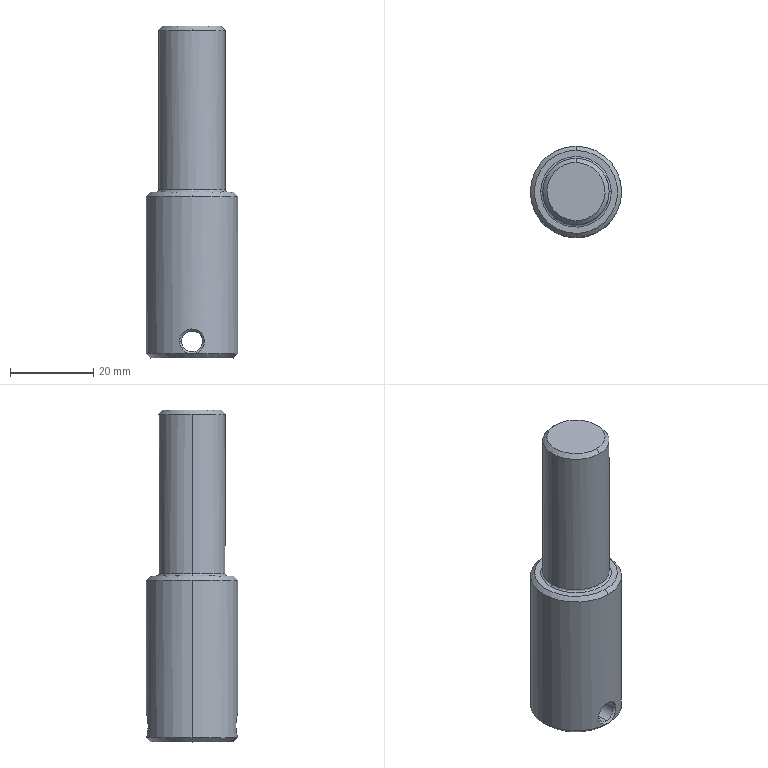Part | SolidWorks | features BaseBody 1 | 1 solid | 21 faces | box 22 x 22 x 80 mm | volume 22726 mm3 | spline 6 | cylinder 6 | cone 6 | plane 3 | commonest cylinder face diameters 5 x2 16 x2 22 x2